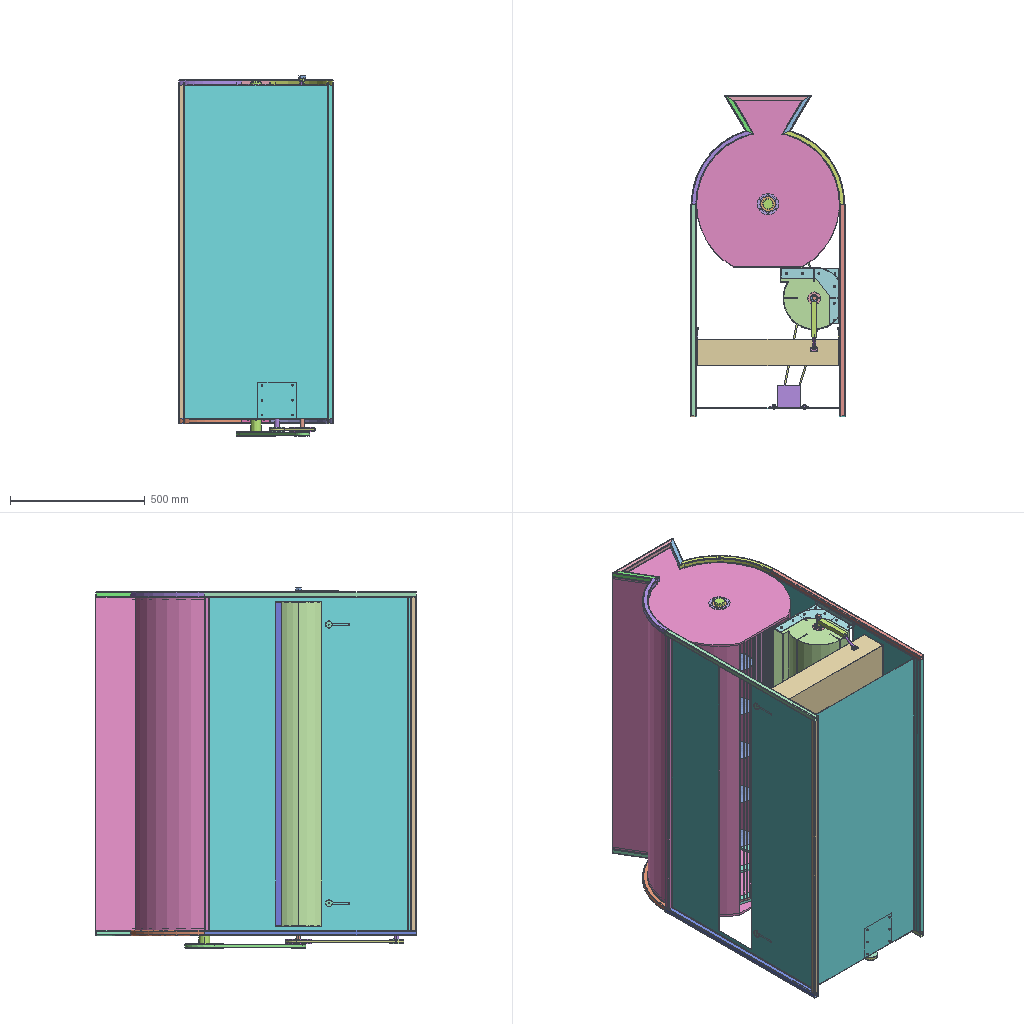Assembly | SolidWorks | 69 different items | 152 placed | box 574 x 1189 x 1337 mm
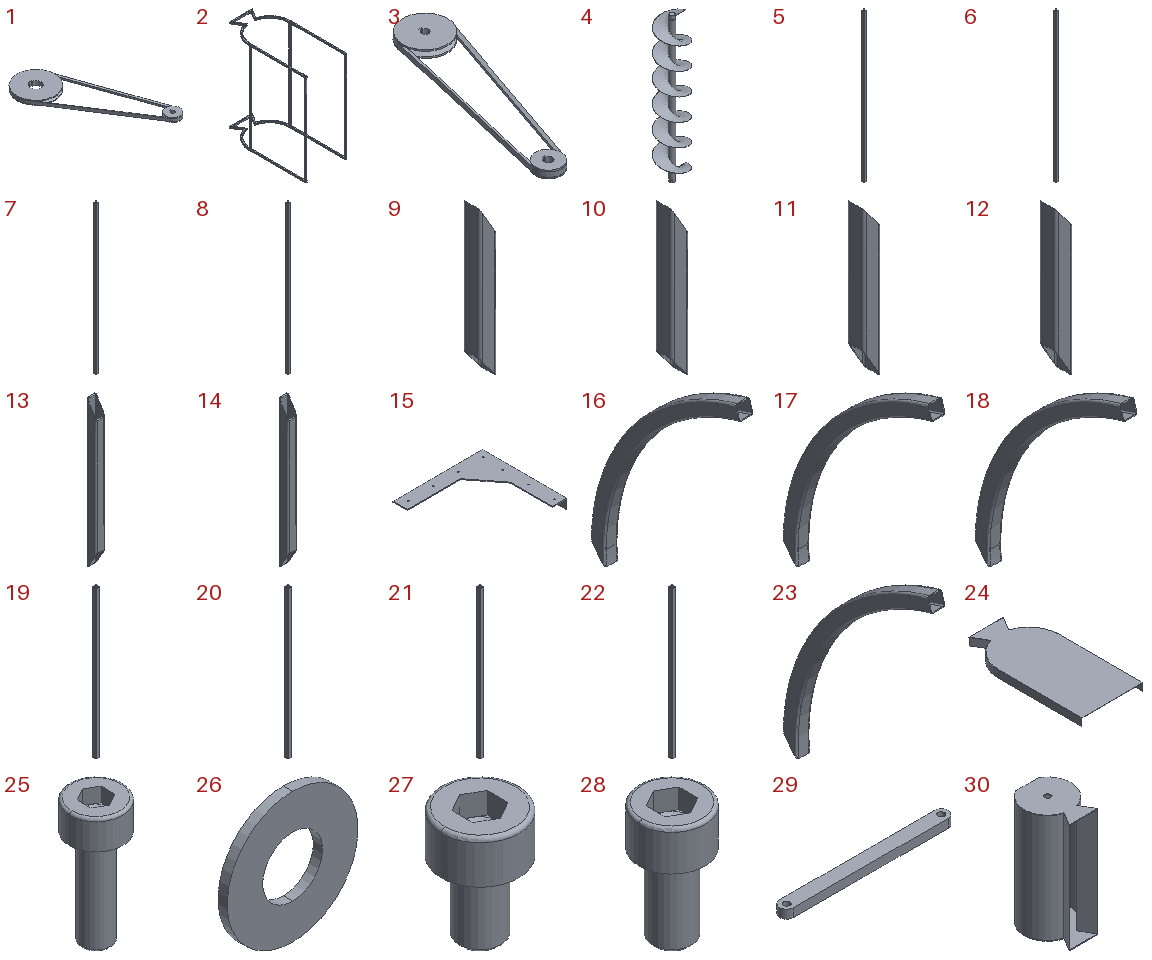Parts list (item | name | quantity | parent item | size | volume | features):
1 | (subassembly) | x1 | - | 271.5 x 449.339 x 16 mm | 287738 mm3 | -
2 | (subassembly) | x1 | - | 574 x 1189 x 1276 mm | 911886 mm3 | -
3 | (subassembly) | x1 | - | 178.368 x 436.001 x 16 mm | 160469 mm3 | -
4 | (subassembly) | x1 | - | 253.758 x 253.748 x 1316 mm | 2925068 mm3 | -
5 | - | x1 | in 2 | 20 x 20 x 1236 mm | 105425 mm3 | features BaseBody 1
6 | - | x1 | in 2 | 20 x 20 x 1236 mm | 105425 mm3 | features BaseBody 1
7 | - | x1 | in 2 | 20 x 20 x 1236 mm | 105425 mm3 | features BaseBody 1
8 | - | x1 | in 2 | 20 x 20 x 1236 mm | 105425 mm3 | features BaseBody 1
9 | - | x1 | in 2 | 20 x 20 x 178.33 mm | 12571 mm3 | features BaseBody 1
10 | - | x1 | in 2 | 20 x 20 x 178.33 mm | 12571 mm3 | features BaseBody 1
11 | - | x1 | in 2 | 20 x 20 x 178.414 mm | 12580 mm3 | features BaseBody 1
12 | - | x1 | in 2 | 20 x 20 x 178.414 mm | 12580 mm3 | features BaseBody 1
13 | - | x1 | in 2 | 20 x 20 x 320.082 mm | 24308 mm3 | features BaseBody 1
14 | - | x1 | in 2 | 20 x 20 x 320.082 mm | 24308 mm3 | features BaseBody 1
15 | - | x1 | - | 215.539 x 201.719 x 23.05 mm | 38142 mm3 | features BaseBody 1
16 | - | x1 | in 2 | 20 x 212.461 x 295.029 mm | 30994 mm3 | features BaseBody 1
17 | - | x1 | in 2 | 20 x 212.905 x 295.178 mm | 31033 mm3 | features BaseBody 1
18 | - | x1 | in 2 | 20 x 212.905 x 295.178 mm | 31033 mm3 | features BaseBody 1
19 | - | x1 | in 2 | 20 x 20 x 786.319 mm | 67070 mm3 | features BaseBody 1
20 | - | x1 | in 2 | 20 x 20 x 786.319 mm | 67070 mm3 | features BaseBody 1
21 | - | x1 | in 2 | 20 x 20 x 786.319 mm | 67070 mm3 | features BaseBody 1
22 | - | x1 | in 2 | 20 x 20 x 786.319 mm | 67070 mm3 | features BaseBody 1
23 | - | x1 | in 2 | 20 x 212.461 x 295.029 mm | 30989 mm3 | features BaseBody 1
24 | - | x2 | - | 578 x 1192 x 70 mm | 1625565 mm3 | features EdgeFlange 5, 3DProfileFeature 2, FlatPattern 1, ICE 1, SMBaseFlange 1, SheetMetal 1
25 | - | x6 | - | 5.5 x 5.5 x 13 mm | 119.572 mm3 | features Fillet 2, ICE 2, Chamfer 1, Revolution 1
26 | - | x26 | - | 7 x 0.5 x 7 mm | 15.221 mm3 | features Extrusion 1
27 | - | x20 | - | 5.5 x 5.5 x 8 mm | 89.884 mm3 | features Fillet 2, ICE 2, Chamfer 1, Revolution 1
28 | - | x6 | - | 10 x 10 x 18 mm | 687.683 mm3 | features Fillet 2, ICE 2, Chamfer 1, Revolution 1
29 | - | x2 | - | 80.131 x 6.513 x 4.119 mm | 2054 mm3 | features BaseBody 1
30 | - | x1 | - | 530 x 635.026 x 1236 mm | 7825793 mm3 | features BaseBody 1
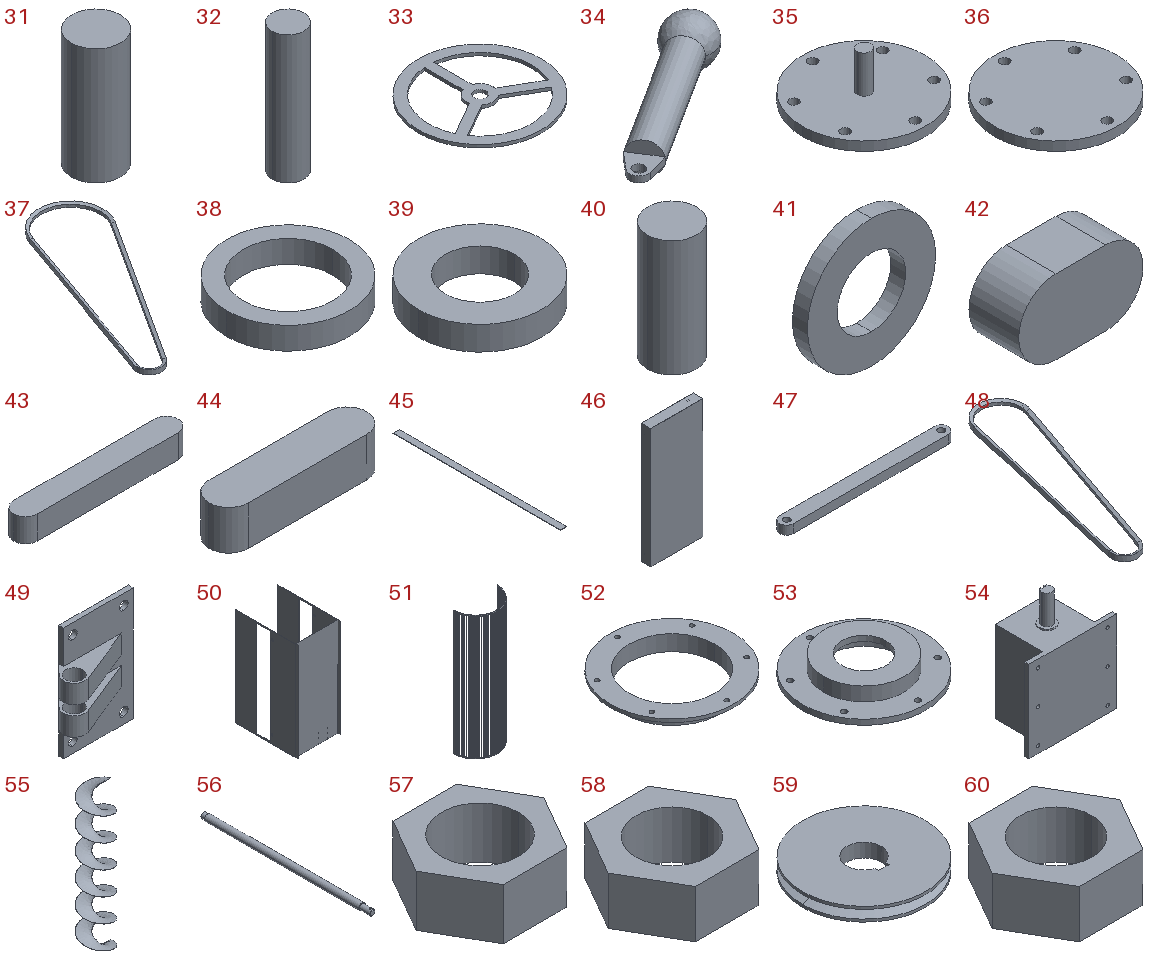31 | - | x2 | - | 3 x 3 x 7.119 mm | 50.318 mm3 | features BaseBody 1
32 | - | x1 | - | 3.663 x 3.663 x 14.762 mm | 155.592 mm3 | features BaseBody 1
33 | - | x2 | - | 420 x 420 x 10 mm | 593937 mm3 | features BaseBody 1
34 | - | x1 | - | 55.474 x 39.094 x 14.478 mm | 4963 mm3 | features BaseBody 1
35 | - | x2 | - | 27.511 x 27.511 x 10.35 mm | 1209 mm3 | features BaseBody 1
36 | - | x2 | - | 27.511 x 27.511 x 10.35 mm | 1209 mm3 | features BaseBody 1
37 | - | x1 | in 1 | 271.5 x 449.339 x 10.319 mm | 52741 mm3 | features BaseBody 1
38 | - | x2 | - | 55 x 55 x 10 mm | 11192 mm3 | features BaseBody 1
39 | - | x2 | - | 26.799 x 26.799 x 5.237 mm | 2029 mm3 | features BaseBody 1
40 | - | x2 | - | 3 x 3 x 7.119 mm | 50.318 mm3 | features BaseBody 1
41 | - | x6 | - | 12 x 1.4 x 12 mm | 113.298 mm3 | features Extrusion 1
42 | - | x1 | - | 20 x 8 x 12 mm | 1673 mm3 | features Extrusion 1
43 | - | x1 | - | 35 x 5 x 5 mm | 848.175 mm3 | features Extrusion 1
44 | - | x1 | - | 20 x 5 x 5 mm | 473.175 mm3 | features Extrusion 1
45 | - | x3 | - | 44.635 x 1200 x 3 mm | 160685 mm3 | features BaseBody 1
46 | - | x1 | - | 521.763 x 96.993 x 1200 mm | 956249 mm3 | features BaseBody 1
47 | - | x2 | - | 80.131 x 6.513 x 4.119 mm | 2054 mm3 | features BaseBody 1
48 | - | x1 | in 3 | 178.368 x 436.001 x 10.319 mm | 47372 mm3 | features BaseBody 1
49 | - | x1 | - | 17.607 x 5.957 x 24.289 mm | 605.772 mm3 | features BaseBody 1
50 | - | x1 | - | 534 x 786.319 x 1236 mm | 4372882 mm3 | features BaseBody 1
51 | - | x1 | - | 420 x 210 x 1200 mm | 419313 mm3 | features BaseBody 1
52 | - | x2 | - | 79 x 79 x 10 mm | 9356 mm3 | features BaseBody 1
53 | - | x2 | - | 47.022 x 47.022 x 7.237 mm | 3944 mm3 | features BaseBody 1
54 | - | x1 | - | 143.331 x 84.235 x 183.45 mm | 1010969 mm3 | features BaseBody 1, ICE 1
55 | - | x1 | in 4 | 253.758 x 253.748 x 1200 mm | 425695 mm3 | features BaseBody 1
56 | - | x1 | in 4 | 50 x 1316 x 50 mm | 2500128 mm3 | features ICE 2, BaseBody 1, Chamfer 1
57 | - | x1 | - | 24.848 x 21.519 x 10 mm | 2243 mm3 | features BaseBody 1
58 | - | x4 | - | 5.314 x 4.602 x 2 mm | 22.552 mm3 | features BaseBody 1
59 | - | x1 | in 1 | 144 x 144 x 16 mm | 211309 mm3 | features ICE 2, BaseBody 1
60 | - | x4 | - | 5.314 x 4.602 x 2 mm | 22.552 mm3 | features BaseBody 1
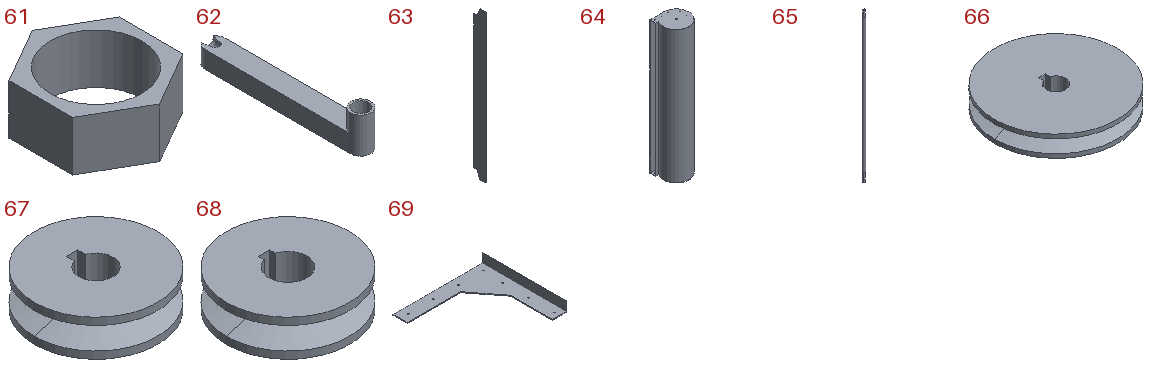61 | - | x2 | - | 4.422 x 5.106 x 2 mm | 12.787 mm3 | features BaseBody 1
62 | - | x1 | - | 18.898 x 156.922 x 33.625 mm | 44298 mm3 | features BaseBody 1
63 | - | x4 | - | 3.795 x 101.02 x 1200 mm | 442400 mm3 | features BaseBody 1
64 | - | x1 | - | 239.936 x 230.88 x 1204 mm | 2000614 mm3 | features BaseBody 1
65 | - | x1 | - | 22.084 x 22.084 x 1336 mm | 483171 mm3 | features BaseBody 1, ICE 1, MoveFace 1
66 | - | x1 | in 3 | 94 x 94 x 16 mm | 89995 mm3 | features ICE 2, BaseBody 1
67 | - | x1 | in 1 | 54 x 54 x 16 mm | 23688 mm3 | features ICE 2, BaseBody 1
68 | - | x1 | in 3 | 54 x 54 x 16 mm | 23103 mm3 | features ICE 2, BaseBody 1
69 | - | x1 | - | 215.539 x 201.719 x 23.05 mm | 38142 mm3 | features BaseBody 1
Mates (type | each side: item.copy, entity, surface, feature):
Concentric | 67.1 edge | 65.1 face cylinder Input1
Concentric | 66.1 face cylinder Input1 | 65.1 face cylinder Input1
Coincident | 68.1 face plane Input1 | 54.1 face plane Input1
Concentric | 50.1 face cylinder Input1 | 54.1 face cylinder Input1
Concentric | 33.1 edge | 30.1 edge
Coincident | 50.1 face plane Input1 | 54.1 face plane Input1
Concentric | 68.1 edge | 54.1 face cylinder Input1
Width | 24.1 face plane Edge-Flange2 | 24.1 face plane Edge-Flange3 | 22.1 face plane Input1 | 21.1 face plane Input1
Coincident | 21.1 face plane Input1 | 24.1 face plane Base-Flange1
Coincident | 21.1 face plane Input1 | 24.1 face plane Edge-Flange3
Width | 24.2 face plane Edge-Flange2 | 24.2 face plane Edge-Flange3 | 19.1 face plane Input1 | 20.1 face plane Input1
Coincident | 19.1 face plane Input1 | 24.2 face plane Edge-Flange2 | 2 times
Concentric | 56.1 face cylinder Input1 | 59.1 edge
Coincident | 56.1 face plane Input1 | 59.1 face plane Input1
Concentric | 33.2 edge | 56.1 face cylinder Input1
Concentric | 56.1 face cylinder Input1 | 52.1 face cylinder Input1 | 3 times
Concentric | 33.1 edge | 56.1 face cylinder Input1
Width | 22.1 face plane Input1 | 20.1 face plane Input1 | 56.1 face plane Input1 | 56.1 face plane Input1
Coincident | 56.1 face plane Input1 | 33.1 face plane Input1
Concentric | 56.1 face cylinder Input1 | 38.1 face cylinder Input1
Coincident | 33.1 face plane Input1 | 38.1 face plane Input1
Coincident | 56.1 face plane Input1 | 33.2 face plane Input1
Coincident | 33.2 face plane Input1 | 38.2 face plane Input1
Concentric | 56.1 face cylinder Input1 | 52.2 face cylinder Input1
Concentric | 56.1 face cylinder Input1 | 38.2 face cylinder Input1
Coincident | 38.2 face plane Input1 | 52.2 face plane Input1
Concentric | 52.2 face cylinder Input1 | 30.1 face cylinder Input1
Coincident | 52.1 face plane Input1 | 38.1 face plane Input1
Concentric | 52.1 face cylinder Input1 | 30.1 face cylinder Input1
Coincident | 64.1 face plane Input1 | 15.1 face plane Input1
Concentric | 64.1 face cylinder Input1 | 15.1 face cylinder Input1 | 2 times
Coincident | 64.1 face plane Input1 | 69.1 face plane Input1
Concentric | 64.1 face cylinder Input1 | 69.1 face cylinder Input1 | 2 times
Width | 64.1 face plane Input1 | 64.1 face plane Input1 | 65.1 face plane Input1 | 65.1 face plane Input1
Concentric | 65.1 face cylinder Input1 | 39.1 face cylinder Input1
Concentric | 65.1 face cylinder Input1 | 53.1 face cylinder Input1
Coincident | 64.1 face plane Input1 | 53.1 face plane Input1
Coincident | 39.1 face plane Input1 | 53.1 face plane Input1
Concentric | 65.1 face cylinder Input1 | 53.2 face cylinder Input1
Coincident | 64.1 face plane Input1 | 53.2 face plane Input1
Concentric | 65.1 face cylinder Input1 | 39.2 face cylinder Input1
Coincident | 53.2 face plane Input1 | 39.2 face plane Input1
Coincident | 54.1 face plane Cut-Extrude1 | 44.1 face plane Boss-Extrude1 | 2 times
Tangent | 54.1 face plane Input1 | 44.1 face cylinder Boss-Extrude1
Concentric | 65.1 face cylinder Input1 | 64.1 face cylinder Input1
Coincident | 65.1 face plane Cut-Extrude1 | 43.1 face plane Boss-Extrude1 | 2 times
Tangent | 65.1 face plane Input1 | 43.1 face cylinder Boss-Extrude1
Coincident | 56.1 face plane Cut-Extrude1 | 42.1 face plane Boss-Extrude1 | 2 times
Tangent | 56.1 face plane Input1 | 42.1 face cylinder Boss-Extrude1
Concentric | 52.2 face cylinder Input1 | 25.1 face cylinder Revolve1
Concentric | 25.1 face cylinder Revolve1 | 26.1 face cylinder Boss-Extrude1
Coincident | 25.1 face plane Revolve1 | 26.1 face plane Boss-Extrude1
Coincident | 52.2 face plane Input1 | 26.1 face plane Boss-Extrude1
Concentric | 27.1 face cylinder Revolve1 | 26.2 face cylinder Boss-Extrude1
Coincident | 27.1 face plane Revolve1 | 26.2 face plane Boss-Extrude1
Concentric | 15.1 face cylinder Input1 | 27.1 face cylinder Revolve1
Coincident | 15.1 face plane Input1 | 26.2 face plane Boss-Extrude1
Concentric | 27.2 face cylinder Revolve1 | 26.3 face cylinder Boss-Extrude1
Coincident | 27.2 face plane Revolve1 | 26.3 face plane Boss-Extrude1
Concentric | 53.2 face cylinder Input1 | 27.2 face cylinder Revolve1
Coincident | 53.2 face plane Input1 | 26.3 face plane Boss-Extrude1
Concentric | 28.1 face cylinder Revolve1 | 41.1 face cylinder Boss-Extrude1
Coincident | 28.1 face plane Revolve1 | 41.1 face plane Boss-Extrude1
Concentric | 54.1 face cylinder Input1 | 28.1 face cylinder Revolve1
Coincident | 54.1 face plane Input1 | 41.1 face plane Boss-Extrude1
Concentric | 41.2 face cylinder Boss-Extrude1 | 28.2 face cylinder Revolve1
Coincident | 41.2 face plane Boss-Extrude1 | 28.2 face plane Revolve1
Concentric | 54.1 face cylinder Input1 | 28.2 face cylinder Revolve1
Coincident | 54.1 face plane Input1 | 41.2 face plane Boss-Extrude1
Concentric | 50.1 face cylinder Input1 | 28.2 face cylinder Revolve1
Concentric | 27.3 face cylinder Revolve1 | 26.4 face cylinder Boss-Extrude1
Coincident | 27.3 face plane Revolve1 | 26.4 face plane Boss-Extrude1
Concentric | 15.1 face cylinder Input1 | 27.3 face cylinder Revolve1
Coincident | 15.1 face plane Input1 | 26.4 face plane Boss-Extrude1
Concentric | 26.5 face cylinder Boss-Extrude1 | 27.4 face cylinder Revolve1
Coincident | 26.5 face plane Boss-Extrude1 | 27.4 face plane Revolve1
Concentric | 69.1 face cylinder Input1 | 27.4 face cylinder Revolve1
Coincident | 69.1 face plane Input1 | 26.5 face plane Boss-Extrude1
Concentric | 27.5 face cylinder Revolve1 | 26.6 face cylinder Boss-Extrude1
Coincident | 27.5 face plane Revolve1 | 26.6 face plane Boss-Extrude1
Coincident | 69.1 face plane Input1 | 26.6 face plane Boss-Extrude1
Concentric | 69.1 face cylinder Input1 | 27.5 face cylinder Revolve1